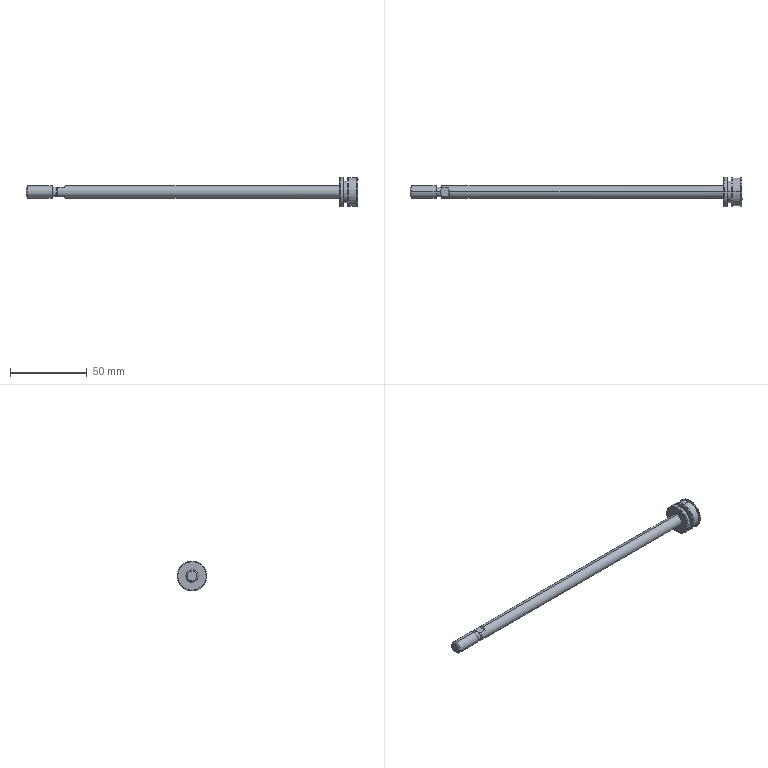Part | STEP file | MI20x125SU-02-cc | 1 solid | 50 faces | box 216.2 x 19.5 x 19.5 mm | volume 13209 mm3 | cylinder 16 | plane 14 | cone 12 | spline 8 | commonest cylinder face diameters 19.5 x6 8 x4 6.4 x2 14 x2 18.3 x2